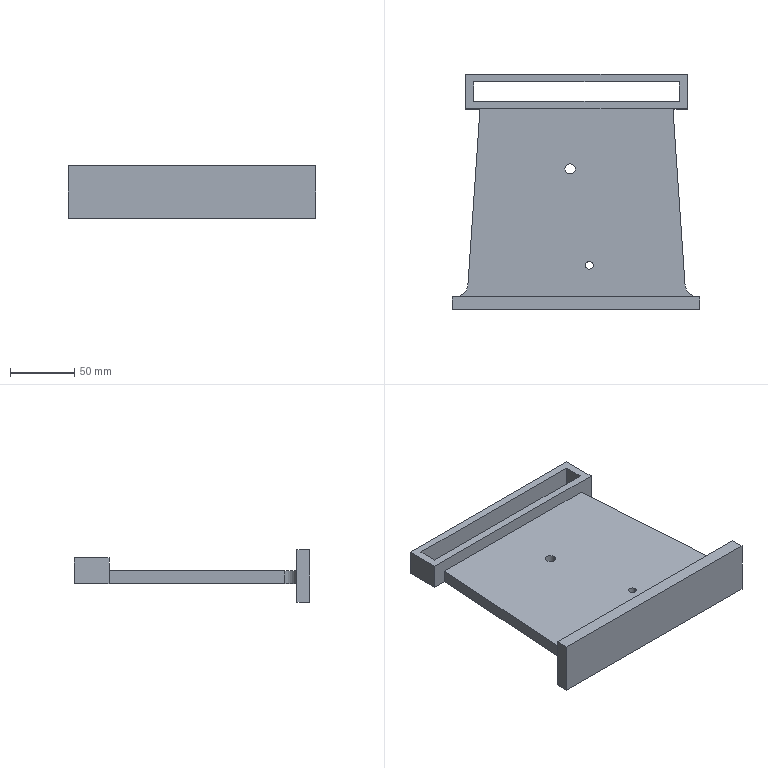Part | SolidWorks | features ICE 2, Extrusion 1, Fillet 1 | 1 solid | 25 faces | box 192.506 x 183 x 41.072 mm | volume 357126 mm3 | plane 19 | cylinder 6 | commonest cylinder face diameters 6 x2 8 x2 20 x2
STEP:
#1=CARTESIAN_POINT('',(76.,99.5,10.));
#2=VERTEX_POINT('',#1);
#3=CARTESIAN_POINT('',(84.,99.5,10.));
#4=VERTEX_POINT('',#3);
#5=CARTESIAN_POINT('',(80.,99.5,10.));
#6=DIRECTION('',(0.,0.,1.));
#7=DIRECTION('',(1.,0.,0.));
#8=AXIS2_PLACEMENT_3D('',#5,#6,#7);
#9=CIRCLE('',#8,4.);
#10=EDGE_CURVE('',#2,#4,#9,.T.);
#11=ORIENTED_EDGE('',*,*,#10,.T.);
#12=CARTESIAN_POINT('',(84.,99.5,0.));
#13=VERTEX_POINT('',#12);
#14=CARTESIAN_POINT('',(84.,99.5,10.));
#15=DIRECTION('',(0.,0.,-1.));
#16=VECTOR('',#15,1000.);
#17=LINE('',#14,#16);
#18=EDGE_CURVE('',#4,#13,#17,.T.);
#19=ORIENTED_EDGE('',*,*,#18,.T.);
#20=CARTESIAN_POINT('',(76.,99.5,0.));
#21=VERTEX_POINT('',#20);
#22=CARTESIAN_POINT('',(80.,99.5,0.));
#23=DIRECTION('',(0.,0.,1.));
#24=DIRECTION('',(1.,0.,0.));
#25=AXIS2_PLACEMENT_3D('',#22,#23,#24);
#26=CIRCLE('',#25,4.);
#27=EDGE_CURVE('',#21,#13,#26,.T.);
#28=ORIENTED_EDGE('',*,*,#27,.F.);
#29=CARTESIAN_POINT('',(76.,99.5,10.));
#30=DIRECTION('',(0.,0.,-1.));
#31=VECTOR('',#30,1000.);
#32=LINE('',#29,#31);
#33=EDGE_CURVE('',#2,#21,#32,.T.);
#34=ORIENTED_EDGE('',*,*,#33,.F.);
#35=EDGE_LOOP('',(#11,#19,#28,#34));
#36=FACE_OUTER_BOUND('',#35,.T.);
#37=CARTESIAN_POINT('',(80.,99.5,10.));
#38=DIRECTION('',(0.,0.,-1.));
#39=DIRECTION('',(-1.,0.,0.));
#40=AXIS2_PLACEMENT_3D('',#37,#38,#39);
#41=CYLINDRICAL_SURFACE('',#40,4.);
#42=ADVANCED_FACE('',(#36),#41,.F.);
#43=CARTESIAN_POINT('',(92.,24.5,10.));
#44=VERTEX_POINT('',#43);
#45=CARTESIAN_POINT('',(98.,24.5,10.));
#46=VERTEX_POINT('',#45);
#47=CARTESIAN_POINT('',(95.,24.5,10.));
#48=DIRECTION('',(0.,0.,1.));
#49=DIRECTION('',(1.,0.,0.));
#50=AXIS2_PLACEMENT_3D('',#47,#48,#49);
#51=CIRCLE('',#50,3.);
#52=EDGE_CURVE('',#44,#46,#51,.T.);
#53=ORIENTED_EDGE('',*,*,#52,.T.);
#54=CARTESIAN_POINT('',(98.,24.5,0.));
#55=VERTEX_POINT('',#54);
#56=CARTESIAN_POINT('',(98.,24.5,10.));
#57=DIRECTION('',(0.,0.,-1.));
#58=VECTOR('',#57,1000.);
#59=LINE('',#56,#58);
#60=EDGE_CURVE('',#46,#55,#59,.T.);
#61=ORIENTED_EDGE('',*,*,#60,.T.);
#62=CARTESIAN_POINT('',(92.,24.5,0.));
#63=VERTEX_POINT('',#62);
#64=CARTESIAN_POINT('',(95.,24.5,0.));
#65=DIRECTION('',(0.,0.,1.));
#66=DIRECTION('',(1.,0.,0.));
#67=AXIS2_PLACEMENT_3D('',#64,#65,#66);
#68=CIRCLE('',#67,3.);
#69=EDGE_CURVE('',#63,#55,#68,.T.);
#70=ORIENTED_EDGE('',*,*,#69,.F.);
#71=CARTESIAN_POINT('',(92.,24.5,10.));
#72=DIRECTION('',(0.,0.,-1.));
#73=VECTOR('',#72,1000.);
#74=LINE('',#71,#73);
#75=EDGE_CURVE('',#44,#63,#74,.T.);
#76=ORIENTED_EDGE('',*,*,#75,.F.);
#77=EDGE_LOOP('',(#53,#61,#70,#76));
#78=FACE_OUTER_BOUND('',#77,.T.);
#79=CARTESIAN_POINT('',(95.,24.5,10.));
#80=DIRECTION('',(0.,0.,-1.));
#81=DIRECTION('',(-1.,0.,0.));
#82=AXIS2_PLACEMENT_3D('',#79,#80,#81);
#83=CYLINDRICAL_SURFACE('',#82,3.);
#84=ADVANCED_FACE('',(#78),#83,.F.);
#85=ORIENTED_EDGE('',*,*,#52,.F.);
#86=CARTESIAN_POINT('',(95.,24.5,10.));
#87=DIRECTION('',(0.,0.,1.));
#88=DIRECTION('',(1.,0.,0.));
#89=AXIS2_PLACEMENT_3D('',#86,#87,#88);
#90=CIRCLE('',#89,3.);
#91=EDGE_CURVE('',#46,#44,#90,.T.);
#92=ORIENTED_EDGE('',*,*,#91,.F.);
#93=EDGE_LOOP('',(#85,#92));
#94=FACE_BOUND('',#93,.T.);
#95=CARTESIAN_POINT('',(10.,146.,10.));
#96=VERTEX_POINT('',#95);
#97=CARTESIAN_POINT('',(0.6381,9.317,10.));
#98=VERTEX_POINT('',#97);
#99=CARTESIAN_POINT('',(10.,146.,10.));
#100=DIRECTION('',(-0.06833,-0.9977,0.));
#101=VECTOR('',#100,1000.);
#102=LINE('',#99,#101);
#103=EDGE_CURVE('',#96,#98,#102,.T.);
#104=ORIENTED_EDGE('',*,*,#103,.T.);
#105=CARTESIAN_POINT('',(-9.338,0.,10.));
#106=VERTEX_POINT('',#105);
#107=CARTESIAN_POINT('',(-9.338,10.,10.));
#108=DIRECTION('',(0.,0.,-1.));
#109=DIRECTION('',(1.,0.,0.));
#110=AXIS2_PLACEMENT_3D('',#107,#108,#109);
#111=CIRCLE('',#110,10.);
#112=EDGE_CURVE('',#98,#106,#111,.T.);
#113=ORIENTED_EDGE('',*,*,#112,.T.);
#114=CARTESIAN_POINT('',(179.338,0.,10.));
#115=VERTEX_POINT('',#114);
#116=CARTESIAN_POINT('',(0.,0.,10.));
#117=DIRECTION('',(1.,0.,0.));
#118=VECTOR('',#117,1000.);
#119=LINE('',#116,#118);
#120=EDGE_CURVE('',#106,#115,#119,.T.);
#121=ORIENTED_EDGE('',*,*,#120,.T.);
#122=CARTESIAN_POINT('',(169.362,9.317,10.));
#123=VERTEX_POINT('',#122);
#124=CARTESIAN_POINT('',(179.338,10.,10.));
#125=DIRECTION('',(0.,0.,-1.));
#126=DIRECTION('',(1.,0.,0.));
#127=AXIS2_PLACEMENT_3D('',#124,#125,#126);
#128=CIRCLE('',#127,10.);
#129=EDGE_CURVE('',#115,#123,#128,.T.);
#130=ORIENTED_EDGE('',*,*,#129,.T.);
#131=CARTESIAN_POINT('',(160.,146.,10.));
#132=VERTEX_POINT('',#131);
#133=CARTESIAN_POINT('',(170.,0.,10.));
#134=DIRECTION('',(-0.06833,0.9977,0.));
#135=VECTOR('',#134,1000.);
#136=LINE('',#133,#135);
#137=EDGE_CURVE('',#123,#132,#136,.T.);
#138=ORIENTED_EDGE('',*,*,#137,.T.);
#139=CARTESIAN_POINT('',(160.,146.,10.));
#140=DIRECTION('',(-1.,0.,0.));
#141=VECTOR('',#140,1000.);
#142=LINE('',#139,#141);
#143=EDGE_CURVE('',#132,#96,#142,.T.);
#144=ORIENTED_EDGE('',*,*,#143,.T.);
#145=EDGE_LOOP('',(#104,#113,#121,#130,#138,#144));
#146=FACE_OUTER_BOUND('',#145,.T.);
#147=ORIENTED_EDGE('',*,*,#10,.F.);
#148=CARTESIAN_POINT('',(80.,99.5,10.));
#149=DIRECTION('',(0.,0.,1.));
#150=DIRECTION('',(1.,0.,0.));
#151=AXIS2_PLACEMENT_3D('',#148,#149,#150);
#152=CIRCLE('',#151,4.);
#153=EDGE_CURVE('',#4,#2,#152,.T.);
#154=ORIENTED_EDGE('',*,*,#153,.F.);
#155=EDGE_LOOP('',(#147,#154));
#156=FACE_BOUND('',#155,.T.);
#157=CARTESIAN_POINT('',(0.,0.,10.));
#158=DIRECTION('',(0.,0.,1.));
#159=DIRECTION('',(1.,0.,0.));
#160=AXIS2_PLACEMENT_3D('',#157,#158,#159);
#161=PLANE('',#160);
#162=ADVANCED_FACE('',(#94,#146,#156),#161,.T.);
#163=CARTESIAN_POINT('',(10.,146.,0.));
#164=VERTEX_POINT('',#163);
#165=CARTESIAN_POINT('',(0.6381,9.317,0.));
#166=VERTEX_POINT('',#165);
#167=CARTESIAN_POINT('',(10.,146.,0.));
#168=DIRECTION('',(-0.06833,-0.9977,0.));
#169=VECTOR('',#168,1000.);
#170=LINE('',#167,#169);
#171=EDGE_CURVE('',#164,#166,#170,.T.);
#172=ORIENTED_EDGE('',*,*,#171,.F.);
#173=CARTESIAN_POINT('',(-1.,146.,0.));
#174=VERTEX_POINT('',#173);
#175=CARTESIAN_POINT('',(-1.,146.,0.));
#176=DIRECTION('',(1.,0.,0.));
#177=VECTOR('',#176,1000.);
#178=LINE('',#175,#177);
#179=EDGE_CURVE('',#174,#164,#178,.T.);
#180=ORIENTED_EDGE('',*,*,#179,.F.);
#181=CARTESIAN_POINT('',(-1.,173.,0.));
#182=VERTEX_POINT('',#181);
#183=CARTESIAN_POINT('',(-1.,173.,0.));
#184=DIRECTION('',(0.,-1.,0.));
#185=VECTOR('',#184,1000.);
#186=LINE('',#183,#185);
#187=EDGE_CURVE('',#182,#174,#186,.T.);
#188=ORIENTED_EDGE('',*,*,#187,.F.);
#189=CARTESIAN_POINT('',(171.,173.,0.));
#190=VERTEX_POINT('',#189);
#191=CARTESIAN_POINT('',(-1.,173.,0.));
#192=DIRECTION('',(-1.,0.,0.));
#193=VECTOR('',#192,1000.);
#194=LINE('',#191,#193);
#195=EDGE_CURVE('',#190,#182,#194,.T.);
#196=ORIENTED_EDGE('',*,*,#195,.F.);
#197=CARTESIAN_POINT('',(171.,146.,0.));
#198=VERTEX_POINT('',#197);
#199=CARTESIAN_POINT('',(171.,173.,0.));
#200=DIRECTION('',(0.,1.,0.));
#201=VECTOR('',#200,1000.);
#202=LINE('',#199,#201);
#203=EDGE_CURVE('',#198,#190,#202,.T.);
#204=ORIENTED_EDGE('',*,*,#203,.F.);
#205=CARTESIAN_POINT('',(160.,146.,0.));
#206=VERTEX_POINT('',#205);
#207=CARTESIAN_POINT('',(-1.,146.,0.));
#208=DIRECTION('',(1.,0.,0.));
#209=VECTOR('',#208,1000.);
#210=LINE('',#207,#209);
#211=EDGE_CURVE('',#206,#198,#210,.T.);
#212=ORIENTED_EDGE('',*,*,#211,.F.);
#213=CARTESIAN_POINT('',(169.362,9.317,0.));
#214=VERTEX_POINT('',#213);
#215=CARTESIAN_POINT('',(170.,0.,0.));
#216=DIRECTION('',(-0.06833,0.9977,0.));
#217=VECTOR('',#216,1000.);
#218=LINE('',#215,#217);
#219=EDGE_CURVE('',#214,#206,#218,.T.);
#220=ORIENTED_EDGE('',*,*,#219,.F.);
#221=CARTESIAN_POINT('',(179.338,0.,0.));
#222=VERTEX_POINT('',#221);
#223=CARTESIAN_POINT('',(179.338,10.,0.));
#224=DIRECTION('',(0.,0.,1.));
#225=DIRECTION('',(1.,0.,0.));
#226=AXIS2_PLACEMENT_3D('',#223,#224,#225);
#227=CIRCLE('',#226,10.);
#228=EDGE_CURVE('',#214,#222,#227,.T.);
#229=ORIENTED_EDGE('',*,*,#228,.T.);
#230=CARTESIAN_POINT('',(-9.338,0.,0.));
#231=VERTEX_POINT('',#230);
#232=CARTESIAN_POINT('',(0.,0.,0.));
#233=DIRECTION('',(1.,0.,0.));
#234=VECTOR('',#233,1000.);
#235=LINE('',#232,#234);
#236=EDGE_CURVE('',#231,#222,#235,.T.);
#237=ORIENTED_EDGE('',*,*,#236,.F.);
#238=CARTESIAN_POINT('',(-9.338,10.,0.));
#239=DIRECTION('',(0.,0.,1.));
#240=DIRECTION('',(1.,0.,0.));
#241=AXIS2_PLACEMENT_3D('',#238,#239,#240);
#242=CIRCLE('',#241,10.);
#243=EDGE_CURVE('',#231,#166,#242,.T.);
#244=ORIENTED_EDGE('',*,*,#243,.T.);
#245=EDGE_LOOP('',(#172,#180,#188,#196,#204,#212,#220,#229,#237,#244));
#246=FACE_OUTER_BOUND('',#245,.T.);
#247=ORIENTED_EDGE('',*,*,#69,.T.);
#248=CARTESIAN_POINT('',(95.,24.5,0.));
#249=DIRECTION('',(0.,0.,1.));
#250=DIRECTION('',(1.,0.,0.));
#251=AXIS2_PLACEMENT_3D('',#248,#249,#250);
#252=CIRCLE('',#251,3.);
#253=EDGE_CURVE('',#55,#63,#252,.T.);
#254=ORIENTED_EDGE('',*,*,#253,.T.);
#255=EDGE_LOOP('',(#247,#254));
#256=FACE_BOUND('',#255,.T.);
#257=ORIENTED_EDGE('',*,*,#27,.T.);
#258=CARTESIAN_POINT('',(80.,99.5,0.));
#259=DIRECTION('',(0.,0.,1.));
#260=DIRECTION('',(1.,0.,0.));
#261=AXIS2_PLACEMENT_3D('',#258,#259,#260);
#262=CIRCLE('',#261,4.);
#263=EDGE_CURVE('',#13,#21,#262,.T.);
#264=ORIENTED_EDGE('',*,*,#263,.T.);
#265=EDGE_LOOP('',(#257,#264));
#266=FACE_BOUND('',#265,.T.);
#267=CARTESIAN_POINT('',(165.,167.,0.));
#268=VERTEX_POINT('',#267);
#269=CARTESIAN_POINT('',(5.,167.,0.));
#270=VERTEX_POINT('',#269);
#271=CARTESIAN_POINT('',(5.,167.,0.));
#272=DIRECTION('',(-1.,0.,0.));
#273=VECTOR('',#272,1000.);
#274=LINE('',#271,#273);
#275=EDGE_CURVE('',#268,#270,#274,.T.);
#276=ORIENTED_EDGE('',*,*,#275,.T.);
#277=CARTESIAN_POINT('',(5.,152.,0.));
#278=VERTEX_POINT('',#277);
#279=CARTESIAN_POINT('',(5.,152.,0.));
#280=DIRECTION('',(0.,-1.,0.));
#281=VECTOR('',#280,1000.);
#282=LINE('',#279,#281);
#283=EDGE_CURVE('',#270,#278,#282,.T.);
#284=ORIENTED_EDGE('',*,*,#283,.T.);
#285=CARTESIAN_POINT('',(165.,152.,0.));
#286=VERTEX_POINT('',#285);
#287=CARTESIAN_POINT('',(5.,152.,0.));
#288=DIRECTION('',(1.,0.,0.));
#289=VECTOR('',#288,1000.);
#290=LINE('',#287,#289);
#291=EDGE_CURVE('',#278,#286,#290,.T.);
#292=ORIENTED_EDGE('',*,*,#291,.T.);
#293=CARTESIAN_POINT('',(165.,152.,0.));
#294=DIRECTION('',(0.,1.,0.));
#295=VECTOR('',#294,1000.);
#296=LINE('',#293,#295);
#297=EDGE_CURVE('',#286,#268,#296,.T.);
#298=ORIENTED_EDGE('',*,*,#297,.T.);
#299=EDGE_LOOP('',(#276,#284,#292,#298));
#300=FACE_BOUND('',#299,.T.);
#301=CARTESIAN_POINT('',(0.,0.,0.));
#302=DIRECTION('',(0.,0.,1.));
#303=DIRECTION('',(1.,0.,0.));
#304=AXIS2_PLACEMENT_3D('',#301,#302,#303);
#305=PLANE('',#304);
#306=ADVANCED_FACE('',(#246,#256,#266,#300),#305,.F.);
#307=ORIENTED_EDGE('',*,*,#171,.T.);
#308=CARTESIAN_POINT('',(0.6381,9.317,10.));
#309=DIRECTION('',(0.,0.,1.));
#310=VECTOR('',#309,1000.);
#311=LINE('',#308,#310);
#312=EDGE_CURVE('',#166,#98,#311,.T.);
#313=ORIENTED_EDGE('',*,*,#312,.T.);
#314=ORIENTED_EDGE('',*,*,#103,.F.);
#315=CARTESIAN_POINT('',(10.,146.,10.));
#316=DIRECTION('',(0.,0.,-1.));
#317=VECTOR('',#316,1000.);
#318=LINE('',#315,#317);
#319=EDGE_CURVE('',#96,#164,#318,.T.);
#320=ORIENTED_EDGE('',*,*,#319,.T.);
#321=EDGE_LOOP('',(#307,#313,#314,#320));
#322=FACE_OUTER_BOUND('',#321,.T.);
#323=CARTESIAN_POINT('',(10.,146.,10.));
#324=DIRECTION('',(0.9977,-0.06833,0.));
#325=DIRECTION('',(0.06833,0.9977,0.));
#326=AXIS2_PLACEMENT_3D('',#323,#324,#325);
#327=PLANE('',#326);
#328=ADVANCED_FACE('',(#322),#327,.F.);
#329=ORIENTED_EDGE('',*,*,#137,.F.);
#330=CARTESIAN_POINT('',(169.362,9.317,0.));
#331=DIRECTION('',(0.,0.,-1.));
#332=VECTOR('',#331,1000.);
#333=LINE('',#330,#332);
#334=EDGE_CURVE('',#123,#214,#333,.T.);
#335=ORIENTED_EDGE('',*,*,#334,.T.);
#336=ORIENTED_EDGE('',*,*,#219,.T.);
#337=CARTESIAN_POINT('',(160.,146.,10.));
#338=DIRECTION('',(0.,0.,-1.));
#339=VECTOR('',#338,1000.);
#340=LINE('',#337,#339);
#341=EDGE_CURVE('',#132,#206,#340,.T.);
#342=ORIENTED_EDGE('',*,*,#341,.F.);
#343=EDGE_LOOP('',(#329,#335,#336,#342));
#344=FACE_OUTER_BOUND('',#343,.T.);
#345=CARTESIAN_POINT('',(170.,0.,10.));
#346=DIRECTION('',(-0.9977,-0.06833,0.));
#347=DIRECTION('',(0.06833,-0.9977,0.));
#348=AXIS2_PLACEMENT_3D('',#345,#346,#347);
#349=PLANE('',#348);
#350=ADVANCED_FACE('',(#344),#349,.F.);
#351=ORIENTED_EDGE('',*,*,#60,.F.);
#352=ORIENTED_EDGE('',*,*,#91,.T.);
#353=ORIENTED_EDGE('',*,*,#75,.T.);
#354=ORIENTED_EDGE('',*,*,#253,.F.);
#355=EDGE_LOOP('',(#351,#352,#353,#354));
#356=FACE_OUTER_BOUND('',#355,.T.);
#357=CARTESIAN_POINT('',(95.,24.5,10.));
#358=DIRECTION('',(0.,0.,-1.));
#359=DIRECTION('',(-1.,0.,0.));
#360=AXIS2_PLACEMENT_3D('',#357,#358,#359);
#361=CYLINDRICAL_SURFACE('',#360,3.);
#362=ADVANCED_FACE('',(#356),#361,.F.);
#363=ORIENTED_EDGE('',*,*,#18,.F.);
#364=ORIENTED_EDGE('',*,*,#153,.T.);
#365=ORIENTED_EDGE('',*,*,#33,.T.);
#366=ORIENTED_EDGE('',*,*,#263,.F.);
#367=EDGE_LOOP('',(#363,#364,#365,#366));
#368=FACE_OUTER_BOUND('',#367,.T.);
#369=CARTESIAN_POINT('',(80.,99.5,10.));
#370=DIRECTION('',(0.,0.,-1.));
#371=DIRECTION('',(-1.,0.,0.));
#372=AXIS2_PLACEMENT_3D('',#369,#370,#371);
#373=CYLINDRICAL_SURFACE('',#372,4.);
#374=ADVANCED_FACE('',(#368),#373,.F.);
#375=CARTESIAN_POINT('',(180.891,0.,-14.617));
#376=VERTEX_POINT('',#375);
#377=CARTESIAN_POINT('',(180.891,0.,26.455));
#378=VERTEX_POINT('',#377);
#379=CARTESIAN_POINT('',(180.891,0.,26.455));
#380=DIRECTION('',(0.,0.,1.));
#381=VECTOR('',#380,1000.);
#382=LINE('',#379,#381);
#383=EDGE_CURVE('',#376,#378,#382,.T.);
#384=ORIENTED_EDGE('',*,*,#383,.F.);
#385=CARTESIAN_POINT('',(-11.615,0.,-14.617));
#386=VERTEX_POINT('',#385);
#387=CARTESIAN_POINT('',(-11.615,0.,-14.617));
#388=DIRECTION('',(1.,0.,0.));
#389=VECTOR('',#388,1000.);
#390=LINE('',#387,#389);
#391=EDGE_CURVE('',#386,#376,#390,.T.);
#392=ORIENTED_EDGE('',*,*,#391,.F.);
#393=CARTESIAN_POINT('',(-11.615,0.,26.455));
#394=VERTEX_POINT('',#393);
#395=CARTESIAN_POINT('',(-11.615,0.,26.455));
#396=DIRECTION('',(0.,0.,-1.));
#397=VECTOR('',#396,1000.);
#398=LINE('',#395,#397);
#399=EDGE_CURVE('',#394,#386,#398,.T.);
#400=ORIENTED_EDGE('',*,*,#399,.F.);
#401=CARTESIAN_POINT('',(-11.615,0.,26.455));
#402=DIRECTION('',(-1.,0.,0.));
#403=VECTOR('',#402,1000.);
#404=LINE('',#401,#403);
#405=EDGE_CURVE('',#378,#394,#404,.T.);
#406=ORIENTED_EDGE('',*,*,#405,.F.);
#407=EDGE_LOOP('',(#384,#392,#400,#406));
#408=FACE_OUTER_BOUND('',#407,.T.);
#409=ORIENTED_EDGE('',*,*,#236,.T.);
#410=CARTESIAN_POINT('',(179.338,0.,10.));
#411=DIRECTION('',(0.,0.,1.));
#412=VECTOR('',#411,1000.);
#413=LINE('',#410,#412);
#414=EDGE_CURVE('',#222,#115,#413,.T.);
#415=ORIENTED_EDGE('',*,*,#414,.T.);
#416=ORIENTED_EDGE('',*,*,#120,.F.);
#417=CARTESIAN_POINT('',(-9.338,0.,0.));
#418=DIRECTION('',(0.,0.,-1.));
#419=VECTOR('',#418,1000.);
#420=LINE('',#417,#419);
#421=EDGE_CURVE('',#106,#231,#420,.T.);
#422=ORIENTED_EDGE('',*,*,#421,.T.);
#423=EDGE_LOOP('',(#409,#415,#416,#422));
#424=FACE_BOUND('',#423,.T.);
#425=CARTESIAN_POINT('',(0.,0.,0.));
#426=DIRECTION('',(0.,-1.,0.));
#427=DIRECTION('',(0.,0.,-1.));
#428=AXIS2_PLACEMENT_3D('',#425,#426,#427);
#429=PLANE('',#428);
#430=ADVANCED_FACE('',(#408,#424),#429,.F.);
#431=ORIENTED_EDGE('',*,*,#383,.T.);
#432=CARTESIAN_POINT('',(180.891,-10.,26.455));
#433=VERTEX_POINT('',#432);
#434=CARTESIAN_POINT('',(180.891,-10.,26.455));
#435=DIRECTION('',(0.,1.,0.));
#436=VECTOR('',#435,1000.);
#437=LINE('',#434,#436);
#438=EDGE_CURVE('',#433,#378,#437,.T.);
#439=ORIENTED_EDGE('',*,*,#438,.F.);
#440=CARTESIAN_POINT('',(180.891,-10.,-14.617));
#441=VERTEX_POINT('',#440);
#442=CARTESIAN_POINT('',(180.891,-10.,26.455));
#443=DIRECTION('',(0.,0.,1.));
#444=VECTOR('',#443,1000.);
#445=LINE('',#442,#444);
#446=EDGE_CURVE('',#441,#433,#445,.T.);
#447=ORIENTED_EDGE('',*,*,#446,.F.);
#448=CARTESIAN_POINT('',(180.891,-10.,-14.617));
#449=DIRECTION('',(0.,1.,0.));
#450=VECTOR('',#449,1000.);
#451=LINE('',#448,#450);
#452=EDGE_CURVE('',#441,#376,#451,.T.);
#453=ORIENTED_EDGE('',*,*,#452,.T.);
#454=EDGE_LOOP('',(#431,#439,#447,#453));
#455=FACE_OUTER_BOUND('',#454,.T.);
#456=CARTESIAN_POINT('',(180.891,-10.,26.455));
#457=DIRECTION('',(-1.,0.,0.));
#458=DIRECTION('',(0.,0.,1.));
#459=AXIS2_PLACEMENT_3D('',#456,#457,#458);
#460=PLANE('',#459);
#461=ADVANCED_FACE('',(#455),#460,.F.);
#462=ORIENTED_EDGE('',*,*,#405,.T.);
#463=CARTESIAN_POINT('',(-11.615,-10.,26.455));
#464=VERTEX_POINT('',#463);
#465=CARTESIAN_POINT('',(-11.615,-10.,26.455));
#466=DIRECTION('',(0.,1.,0.));
#467=VECTOR('',#466,1000.);
#468=LINE('',#465,#467);
#469=EDGE_CURVE('',#464,#394,#468,.T.);
#470=ORIENTED_EDGE('',*,*,#469,.F.);
#471=CARTESIAN_POINT('',(-11.615,-10.,26.455));
#472=DIRECTION('',(-1.,0.,0.));
#473=VECTOR('',#472,1000.);
#474=LINE('',#471,#473);
#475=EDGE_CURVE('',#433,#464,#474,.T.);
#476=ORIENTED_EDGE('',*,*,#475,.F.);
#477=ORIENTED_EDGE('',*,*,#438,.T.);
#478=EDGE_LOOP('',(#462,#470,#476,#477));
#479=FACE_OUTER_BOUND('',#478,.T.);
#480=CARTESIAN_POINT('',(-11.615,-10.,26.455));
#481=DIRECTION('',(0.,0.,-1.));
#482=DIRECTION('',(-1.,0.,0.));
#483=AXIS2_PLACEMENT_3D('',#480,#481,#482);
#484=PLANE('',#483);
#485=ADVANCED_FACE('',(#479),#484,.F.);
#486=ORIENTED_EDGE('',*,*,#399,.T.);
#487=CARTESIAN_POINT('',(-11.615,-10.,-14.617));
#488=VERTEX_POINT('',#487);
#489=CARTESIAN_POINT('',(-11.615,-10.,-14.617));
#490=DIRECTION('',(0.,1.,0.));
#491=VECTOR('',#490,1000.);
#492=LINE('',#489,#491);
#493=EDGE_CURVE('',#488,#386,#492,.T.);
#494=ORIENTED_EDGE('',*,*,#493,.F.);
#495=CARTESIAN_POINT('',(-11.615,-10.,26.455));
#496=DIRECTION('',(0.,0.,-1.));
#497=VECTOR('',#496,1000.);
#498=LINE('',#495,#497);
#499=EDGE_CURVE('',#464,#488,#498,.T.);
#500=ORIENTED_EDGE('',*,*,#499,.F.);
#501=ORIENTED_EDGE('',*,*,#469,.T.);
#502=EDGE_LOOP('',(#486,#494,#500,#501));
#503=FACE_OUTER_BOUND('',#502,.T.);
#504=CARTESIAN_POINT('',(-11.615,-10.,26.455));
#505=DIRECTION('',(1.,0.,0.));
#506=DIRECTION('',(0.,0.,-1.));
#507=AXIS2_PLACEMENT_3D('',#504,#505,#506);
#508=PLANE('',#507);
#509=ADVANCED_FACE('',(#503),#508,.F.);
#510=ORIENTED_EDGE('',*,*,#391,.T.);
#511=ORIENTED_EDGE('',*,*,#452,.F.);
#512=CARTESIAN_POINT('',(-11.615,-10.,-14.617));
#513=DIRECTION('',(1.,0.,0.));
#514=VECTOR('',#513,1000.);
#515=LINE('',#512,#514);
#516=EDGE_CURVE('',#488,#441,#515,.T.);
#517=ORIENTED_EDGE('',*,*,#516,.F.);
#518=ORIENTED_EDGE('',*,*,#493,.T.);
#519=EDGE_LOOP('',(#510,#511,#517,#518));
#520=FACE_OUTER_BOUND('',#519,.T.);
#521=CARTESIAN_POINT('',(-11.615,-10.,-14.617));
#522=DIRECTION('',(0.,0.,1.));
#523=DIRECTION('',(1.,0.,0.));
#524=AXIS2_PLACEMENT_3D('',#521,#522,#523);
#525=PLANE('',#524);
#526=ADVANCED_FACE('',(#520),#525,.F.);
#527=ORIENTED_EDGE('',*,*,#446,.T.);
#528=ORIENTED_EDGE('',*,*,#475,.T.);
#529=ORIENTED_EDGE('',*,*,#499,.T.);
#530=ORIENTED_EDGE('',*,*,#516,.T.);
#531=EDGE_LOOP('',(#527,#528,#529,#530));
#532=FACE_OUTER_BOUND('',#531,.T.);
#533=CARTESIAN_POINT('',(0.,-10.,0.));
#534=DIRECTION('',(0.,-1.,0.));
#535=DIRECTION('',(0.,0.,-1.));
#536=AXIS2_PLACEMENT_3D('',#533,#534,#535);
#537=PLANE('',#536);
#538=ADVANCED_FACE('',(#532),#537,.T.);
#539=ORIENTED_EDGE('',*,*,#129,.F.);
#540=ORIENTED_EDGE('',*,*,#414,.F.);
#541=ORIENTED_EDGE('',*,*,#228,.F.);
#542=ORIENTED_EDGE('',*,*,#334,.F.);
#543=EDGE_LOOP('',(#539,#540,#541,#542));
#544=FACE_OUTER_BOUND('',#543,.T.);
#545=CARTESIAN_POINT('',(179.338,10.,10.));
#546=DIRECTION('',(0.,0.,1.));
#547=DIRECTION('',(1.,0.,0.));
#548=AXIS2_PLACEMENT_3D('',#545,#546,#547);
#549=CYLINDRICAL_SURFACE('',#548,10.);
#550=ADVANCED_FACE('',(#544),#549,.F.);
#551=ORIENTED_EDGE('',*,*,#112,.F.);
#552=ORIENTED_EDGE('',*,*,#312,.F.);
#553=ORIENTED_EDGE('',*,*,#243,.F.);
#554=ORIENTED_EDGE('',*,*,#421,.F.);
#555=EDGE_LOOP('',(#551,#552,#553,#554));
#556=FACE_OUTER_BOUND('',#555,.T.);
#557=CARTESIAN_POINT('',(-9.338,10.,0.));
#558=DIRECTION('',(0.,0.,1.));
#559=DIRECTION('',(1.,0.,0.));
#560=AXIS2_PLACEMENT_3D('',#557,#558,#559);
#561=CYLINDRICAL_SURFACE('',#560,10.);
#562=ADVANCED_FACE('',(#556),#561,.F.);
#563=ORIENTED_EDGE('',*,*,#319,.F.);
#564=ORIENTED_EDGE('',*,*,#143,.F.);
#565=ORIENTED_EDGE('',*,*,#341,.T.);
#566=ORIENTED_EDGE('',*,*,#211,.T.);
#567=CARTESIAN_POINT('',(171.,146.,20.));
#568=VERTEX_POINT('',#567);
#569=CARTESIAN_POINT('',(171.,146.,0.));
#570=DIRECTION('',(0.,0.,1.));
#571=VECTOR('',#570,1000.);
#572=LINE('',#569,#571);
#573=EDGE_CURVE('',#198,#568,#572,.T.);
#574=ORIENTED_EDGE('',*,*,#573,.T.);
#575=CARTESIAN_POINT('',(-1.,146.,20.));
#576=VERTEX_POINT('',#575);
#577=CARTESIAN_POINT('',(-1.,146.,20.));
#578=DIRECTION('',(1.,0.,0.));
#579=VECTOR('',#578,1000.);
#580=LINE('',#577,#579);
#581=EDGE_CURVE('',#576,#568,#580,.T.);
#582=ORIENTED_EDGE('',*,*,#581,.F.);
#583=CARTESIAN_POINT('',(-1.,146.,0.));
#584=DIRECTION('',(0.,0.,1.));
#585=VECTOR('',#584,1000.);
#586=LINE('',#583,#585);
#587=EDGE_CURVE('',#174,#576,#586,.T.);
#588=ORIENTED_EDGE('',*,*,#587,.F.);
#589=ORIENTED_EDGE('',*,*,#179,.T.);
#590=EDGE_LOOP('',(#563,#564,#565,#566,#574,#582,#588,#589));
#591=FACE_OUTER_BOUND('',#590,.T.);
#592=CARTESIAN_POINT('',(-1.,146.,0.));
#593=DIRECTION('',(0.,-1.,0.));
#594=DIRECTION('',(0.,0.,-1.));
#595=AXIS2_PLACEMENT_3D('',#592,#593,#594);
#596=PLANE('',#595);
#597=ADVANCED_FACE('',(#591),#596,.T.);
#598=CARTESIAN_POINT('',(-1.,173.,20.));
#599=VERTEX_POINT('',#598);
#600=CARTESIAN_POINT('',(-1.,173.,20.));
#601=DIRECTION('',(0.,-1.,0.));
#602=VECTOR('',#601,1000.);
#603=LINE('',#600,#602);
#604=EDGE_CURVE('',#599,#576,#603,.T.);
#605=ORIENTED_EDGE('',*,*,#604,.F.);
#606=CARTESIAN_POINT('',(-1.,173.,0.));
#607=DIRECTION('',(0.,0.,1.));
#608=VECTOR('',#607,1000.);
#609=LINE('',#606,#608);
#610=EDGE_CURVE('',#182,#599,#609,.T.);
#611=ORIENTED_EDGE('',*,*,#610,.F.);
#612=ORIENTED_EDGE('',*,*,#187,.T.);
#613=ORIENTED_EDGE('',*,*,#587,.T.);
#614=EDGE_LOOP('',(#605,#611,#612,#613));
#615=FACE_OUTER_BOUND('',#614,.T.);
#616=CARTESIAN_POINT('',(-1.,173.,0.));
#617=DIRECTION('',(-1.,0.,0.));
#618=DIRECTION('',(0.,-1.,0.));
#619=AXIS2_PLACEMENT_3D('',#616,#617,#618);
#620=PLANE('',#619);
#621=ADVANCED_FACE('',(#615),#620,.T.);
#622=CARTESIAN_POINT('',(171.,173.,20.));
#623=VERTEX_POINT('',#622);
#624=CARTESIAN_POINT('',(-1.,173.,20.));
#625=DIRECTION('',(-1.,0.,0.));
#626=VECTOR('',#625,1000.);
#627=LINE('',#624,#626);
#628=EDGE_CURVE('',#623,#599,#627,.T.);
#629=ORIENTED_EDGE('',*,*,#628,.F.);
#630=CARTESIAN_POINT('',(171.,173.,0.));
#631=DIRECTION('',(0.,0.,1.));
#632=VECTOR('',#631,1000.);
#633=LINE('',#630,#632);
#634=EDGE_CURVE('',#190,#623,#633,.T.);
#635=ORIENTED_EDGE('',*,*,#634,.F.);
#636=ORIENTED_EDGE('',*,*,#195,.T.);
#637=ORIENTED_EDGE('',*,*,#610,.T.);
#638=EDGE_LOOP('',(#629,#635,#636,#637));
#639=FACE_OUTER_BOUND('',#638,.T.);
#640=CARTESIAN_POINT('',(-1.,173.,0.));
#641=DIRECTION('',(0.,1.,0.));
#642=DIRECTION('',(0.,0.,1.));
#643=AXIS2_PLACEMENT_3D('',#640,#641,#642);
#644=PLANE('',#643);
#645=ADVANCED_FACE('',(#639),#644,.T.);
#646=CARTESIAN_POINT('',(171.,173.,20.));
#647=DIRECTION('',(0.,1.,0.));
#648=VECTOR('',#647,1000.);
#649=LINE('',#646,#648);
#650=EDGE_CURVE('',#568,#623,#649,.T.);
#651=ORIENTED_EDGE('',*,*,#650,.F.);
#652=ORIENTED_EDGE('',*,*,#573,.F.);
#653=ORIENTED_EDGE('',*,*,#203,.T.);
#654=ORIENTED_EDGE('',*,*,#634,.T.);
#655=EDGE_LOOP('',(#651,#652,#653,#654));
#656=FACE_OUTER_BOUND('',#655,.T.);
#657=CARTESIAN_POINT('',(171.,173.,0.));
#658=DIRECTION('',(1.,0.,0.));
#659=DIRECTION('',(0.,0.,-1.));
#660=AXIS2_PLACEMENT_3D('',#657,#658,#659);
#661=PLANE('',#660);
#662=ADVANCED_FACE('',(#656),#661,.T.);
#663=CARTESIAN_POINT('',(5.,167.,20.));
#664=VERTEX_POINT('',#663);
#665=CARTESIAN_POINT('',(5.,152.,20.));
#666=VERTEX_POINT('',#665);
#667=CARTESIAN_POINT('',(5.,152.,20.));
#668=DIRECTION('',(0.,-1.,0.));
#669=VECTOR('',#668,1000.);
#670=LINE('',#667,#669);
#671=EDGE_CURVE('',#664,#666,#670,.T.);
#672=ORIENTED_EDGE('',*,*,#671,.F.);
#673=CARTESIAN_POINT('',(165.,167.,20.));
#674=VERTEX_POINT('',#673);
#675=CARTESIAN_POINT('',(5.,167.,20.));
#676=DIRECTION('',(-1.,0.,0.));
#677=VECTOR('',#676,1000.);
#678=LINE('',#675,#677);
#679=EDGE_CURVE('',#674,#664,#678,.T.);
#680=ORIENTED_EDGE('',*,*,#679,.F.);
#681=CARTESIAN_POINT('',(165.,152.,20.));
#682=VERTEX_POINT('',#681);
#683=CARTESIAN_POINT('',(165.,152.,20.));
#684=DIRECTION('',(0.,1.,0.));
#685=VECTOR('',#684,1000.);
#686=LINE('',#683,#685);
#687=EDGE_CURVE('',#682,#674,#686,.T.);
#688=ORIENTED_EDGE('',*,*,#687,.F.);
#689=CARTESIAN_POINT('',(5.,152.,20.));
#690=DIRECTION('',(1.,0.,0.));
#691=VECTOR('',#690,1000.);
#692=LINE('',#689,#691);
#693=EDGE_CURVE('',#666,#682,#692,.T.);
#694=ORIENTED_EDGE('',*,*,#693,.F.);
#695=EDGE_LOOP('',(#672,#680,#688,#694));
#696=FACE_BOUND('',#695,.T.);
#697=ORIENTED_EDGE('',*,*,#604,.T.);
#698=ORIENTED_EDGE('',*,*,#581,.T.);
#699=ORIENTED_EDGE('',*,*,#650,.T.);
#700=ORIENTED_EDGE('',*,*,#628,.T.);
#701=EDGE_LOOP('',(#697,#698,#699,#700));
#702=FACE_OUTER_BOUND('',#701,.T.);
#703=CARTESIAN_POINT('',(0.,0.,20.));
#704=DIRECTION('',(0.,0.,1.));
#705=DIRECTION('',(1.,0.,0.));
#706=AXIS2_PLACEMENT_3D('',#703,#704,#705);
#707=PLANE('',#706);
#708=ADVANCED_FACE('',(#696,#702),#707,.T.);
#709=ORIENTED_EDGE('',*,*,#671,.T.);
#710=CARTESIAN_POINT('',(5.,152.,0.));
#711=DIRECTION('',(0.,0.,1.));
#712=VECTOR('',#711,1000.);
#713=LINE('',#710,#712);
#714=EDGE_CURVE('',#278,#666,#713,.T.);
#715=ORIENTED_EDGE('',*,*,#714,.F.);
#716=ORIENTED_EDGE('',*,*,#283,.F.);
#717=CARTESIAN_POINT('',(5.,167.,0.));
#718=DIRECTION('',(0.,0.,1.));
#719=VECTOR('',#718,1000.);
#720=LINE('',#717,#719);
#721=EDGE_CURVE('',#270,#664,#720,.T.);
#722=ORIENTED_EDGE('',*,*,#721,.T.);
#723=EDGE_LOOP('',(#709,#715,#716,#722));
#724=FACE_OUTER_BOUND('',#723,.T.);
#725=CARTESIAN_POINT('',(5.,152.,0.));
#726=DIRECTION('',(-1.,0.,0.));
#727=DIRECTION('',(0.,0.,1.));
#728=AXIS2_PLACEMENT_3D('',#725,#726,#727);
#729=PLANE('',#728);
#730=ADVANCED_FACE('',(#724),#729,.F.);
#731=ORIENTED_EDGE('',*,*,#679,.T.);
#732=ORIENTED_EDGE('',*,*,#721,.F.);
#733=ORIENTED_EDGE('',*,*,#275,.F.);
#734=CARTESIAN_POINT('',(165.,167.,0.));
#735=DIRECTION('',(0.,0.,1.));
#736=VECTOR('',#735,1000.);
#737=LINE('',#734,#736);
#738=EDGE_CURVE('',#268,#674,#737,.T.);
#739=ORIENTED_EDGE('',*,*,#738,.T.);
#740=EDGE_LOOP('',(#731,#732,#733,#739));
#741=FACE_OUTER_BOUND('',#740,.T.);
#742=CARTESIAN_POINT('',(5.,167.,0.));
#743=DIRECTION('',(0.,1.,0.));
#744=DIRECTION('',(0.,0.,1.));
#745=AXIS2_PLACEMENT_3D('',#742,#743,#744);
#746=PLANE('',#745);
#747=ADVANCED_FACE('',(#741),#746,.F.);
#748=ORIENTED_EDGE('',*,*,#687,.T.);
#749=ORIENTED_EDGE('',*,*,#738,.F.);
#750=ORIENTED_EDGE('',*,*,#297,.F.);
#751=CARTESIAN_POINT('',(165.,152.,0.));
#752=DIRECTION('',(0.,0.,1.));
#753=VECTOR('',#752,1000.);
#754=LINE('',#751,#753);
#755=EDGE_CURVE('',#286,#682,#754,.T.);
#756=ORIENTED_EDGE('',*,*,#755,.T.);
#757=EDGE_LOOP('',(#748,#749,#750,#756));
#758=FACE_OUTER_BOUND('',#757,.T.);
#759=CARTESIAN_POINT('',(165.,152.,0.));
#760=DIRECTION('',(1.,0.,0.));
#761=DIRECTION('',(0.,0.,-1.));
#762=AXIS2_PLACEMENT_3D('',#759,#760,#761);
#763=PLANE('',#762);
#764=ADVANCED_FACE('',(#758),#763,.F.);
#765=ORIENTED_EDGE('',*,*,#693,.T.);
#766=ORIENTED_EDGE('',*,*,#755,.F.);
#767=ORIENTED_EDGE('',*,*,#291,.F.);
#768=ORIENTED_EDGE('',*,*,#714,.T.);
#769=EDGE_LOOP('',(#765,#766,#767,#768));
#770=FACE_OUTER_BOUND('',#769,.T.);
#771=CARTESIAN_POINT('',(5.,152.,0.));
#772=DIRECTION('',(0.,-1.,0.));
#773=DIRECTION('',(0.,0.,-1.));
#774=AXIS2_PLACEMENT_3D('',#771,#772,#773);
#775=PLANE('',#774);
#776=ADVANCED_FACE('',(#770),#775,.F.);
#777=CLOSED_SHELL('',(#42,#84,#162,#306,#328,#350,#362,#374,#430,#461,#485,#509,#526,#538,#550,#562,#597,#621,#645,#662,#708,#730,#747,#764,#776));
#778=MANIFOLD_SOLID_BREP('',#777);
#779=CARTESIAN_POINT('',(0.,0.,0.));
#780=DIRECTION('',(0.,0.,1.));
#781=DIRECTION('',(1.,0.,0.));
#782=AXIS2_PLACEMENT_3D('',#779,#780,#781);
#783=(LENGTH_UNIT()NAMED_UNIT(*)SI_UNIT(.MILLI.,.METRE.));
#784=UNCERTAINTY_MEASURE_WITH_UNIT(LENGTH_MEASURE(0.00001),#783,'','');
#785=(NAMED_UNIT(*)PLANE_ANGLE_UNIT()SI_UNIT($,.RADIAN.));
#786=(NAMED_UNIT(*)SI_UNIT($,.STERADIAN.)SOLID_ANGLE_UNIT());
#787=(GEOMETRIC_REPRESENTATION_CONTEXT(3)GLOBAL_UNCERTAINTY_ASSIGNED_CONTEXT((#784))GLOBAL_UNIT_ASSIGNED_CONTEXT((#783,#785,#786))REPRESENTATION_CONTEXT('',''));
#788=ADVANCED_BREP_SHAPE_REPRESENTATION('',(#778,#782),#787);